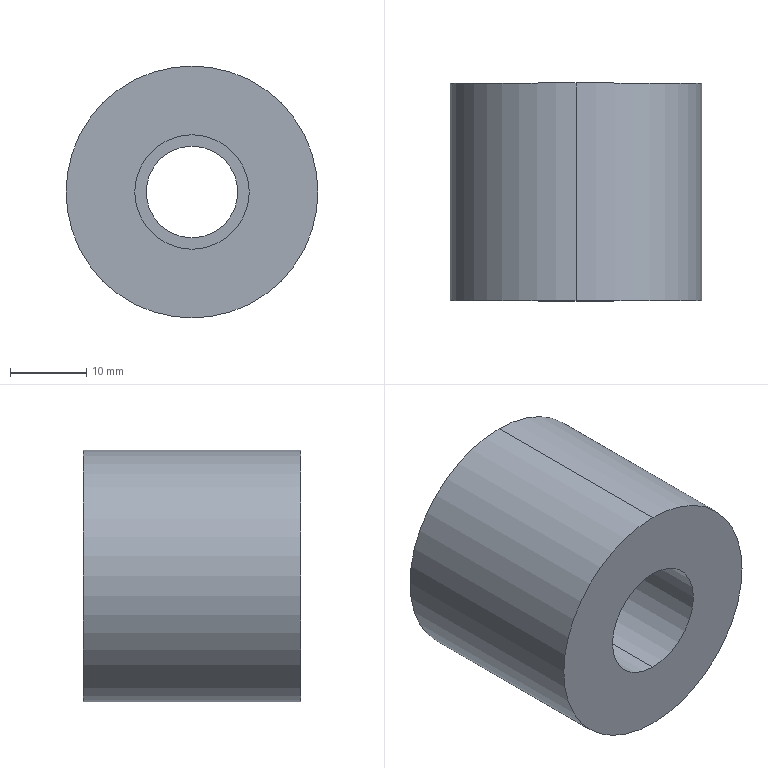Part | STEP file | PN_0065 single diaphragm coupling | 1 solid | 9 faces | box 33 x 28.5 x 33 mm | volume 20198 mm3 | cylinder 6 | plane 3 | commonest cylinder face diameters 12 x2 15 x2 33 x2
STEP:
#1=CARTESIAN_POINT('',(0.,0.,0.));
#2=DIRECTION('',(0.,0.,1.));
#3=DIRECTION('',(1.,0.,0.));
#4=AXIS2_PLACEMENT_3D('',#1,#2,#3);
#5=CARTESIAN_POINT('',(0.,15.,-7.5));
#6=VERTEX_POINT('',#5);
#7=CARTESIAN_POINT('',(0.,0.,-7.5));
#8=VERTEX_POINT('',#7);
#9=CARTESIAN_POINT('',(0.,15.,-7.5));
#10=DIRECTION('',(0.,-1.,0.));
#11=VECTOR('',#10,1.);
#12=LINE('',#9,#11);
#13=CARTESIAN_POINT('',(0.,15.,0.));
#14=DIRECTION('',(0.,-1.,0.));
#15=DIRECTION('',(0.,0.,-1.));
#16=AXIS2_PLACEMENT_3D('',#13,#14,#15);
#17=CYLINDRICAL_SURFACE('',#16,7.5);
#18=CARTESIAN_POINT('',(6.283,0.));
#19=DIRECTION('',(0.,1.));
#20=VECTOR('',#19,1.);
#21=LINE('',#18,#20);
#22=(GEOMETRIC_REPRESENTATION_CONTEXT(2)PARAMETRIC_REPRESENTATION_CONTEXT()REPRESENTATION_CONTEXT('',''));
#23=DEFINITIONAL_REPRESENTATION('',(#21),#22);
#24=PCURVE('',#17,#23);
#25=CARTESIAN_POINT('',(0.,15.,0.));
#26=DIRECTION('',(0.,-1.,0.));
#27=DIRECTION('',(0.,0.,-1.));
#28=AXIS2_PLACEMENT_3D('',#25,#26,#27);
#29=CYLINDRICAL_SURFACE('',#28,7.5);
#30=CARTESIAN_POINT('',(0.,0.));
#31=DIRECTION('',(0.,1.));
#32=VECTOR('',#31,1.);
#33=LINE('',#30,#32);
#34=(GEOMETRIC_REPRESENTATION_CONTEXT(2)PARAMETRIC_REPRESENTATION_CONTEXT()REPRESENTATION_CONTEXT('',''));
#35=DEFINITIONAL_REPRESENTATION('',(#33),#34);
#36=PCURVE('',#29,#35);
#37=SURFACE_CURVE('',#12,(#24,#36),.PCURVE_S1.);
#38=EDGE_CURVE('',#6,#8,#37,.T.);
#39=ORIENTED_EDGE('',*,*,#38,.T.);
#40=CARTESIAN_POINT('',(0.,0.,7.5));
#41=VERTEX_POINT('',#40);
#42=CARTESIAN_POINT('',(0.,0.,0.));
#43=DIRECTION('',(0.,-1.,0.));
#44=DIRECTION('',(0.,0.,-1.));
#45=AXIS2_PLACEMENT_3D('',#42,#43,#44);
#46=CIRCLE('',#45,7.5);
#47=CARTESIAN_POINT('',(0.,15.));
#48=DIRECTION('',(1.,0.));
#49=VECTOR('',#48,1.);
#50=LINE('',#47,#49);
#51=(GEOMETRIC_REPRESENTATION_CONTEXT(2)PARAMETRIC_REPRESENTATION_CONTEXT()REPRESENTATION_CONTEXT('',''));
#52=DEFINITIONAL_REPRESENTATION('',(#50),#51);
#53=PCURVE('',#17,#52);
#54=CARTESIAN_POINT('',(0.,0.,0.));
#55=DIRECTION('',(0.,1.,0.));
#56=DIRECTION('',(0.,0.,1.));
#57=AXIS2_PLACEMENT_3D('',#54,#55,#56);
#58=PLANE('',#57);
#59=CARTESIAN_POINT('',(-7.5,0.));
#60=CARTESIAN_POINT('',(-7.5,12.99));
#61=CARTESIAN_POINT('',(3.75,6.495));
#62=CARTESIAN_POINT('',(15.,0.));
#63=CARTESIAN_POINT('',(3.75,-6.495));
#64=CARTESIAN_POINT('',(-7.5,-12.99));
#65=CARTESIAN_POINT('',(-7.5,0.));
#66=(BOUNDED_CURVE()B_SPLINE_CURVE(2,(#59,#60,#61,#62,#63,#64,#65),.UNSPECIFIED.,.T.,.F.)B_SPLINE_CURVE_WITH_KNOTS((1,2,2,2,2,1),(-2.094,0.,2.094,4.189,6.283,8.378),.UNSPECIFIED.)CURVE()GEOMETRIC_REPRESENTATION_ITEM()RATIONAL_B_SPLINE_CURVE((1.,0.5,1.,0.5,1.,0.5,1.))REPRESENTATION_ITEM(''));
#67=(GEOMETRIC_REPRESENTATION_CONTEXT(2)PARAMETRIC_REPRESENTATION_CONTEXT()REPRESENTATION_CONTEXT('',''));
#68=DEFINITIONAL_REPRESENTATION('',(#66),#67);
#69=PCURVE('',#58,#68);
#70=SURFACE_CURVE('',#46,(#53,#69),.PCURVE_S1.);
#71=EDGE_CURVE('',#41,#8,#70,.T.);
#72=ORIENTED_EDGE('',*,*,#71,.F.);
#73=CARTESIAN_POINT('',(0.,15.,7.5));
#74=VERTEX_POINT('',#73);
#75=CARTESIAN_POINT('',(0.,15.,7.5));
#76=DIRECTION('',(0.,-1.,0.));
#77=VECTOR('',#76,1.);
#78=LINE('',#75,#77);
#79=CARTESIAN_POINT('',(3.142,0.));
#80=DIRECTION('',(0.,1.));
#81=VECTOR('',#80,1.);
#82=LINE('',#79,#81);
#83=(GEOMETRIC_REPRESENTATION_CONTEXT(2)PARAMETRIC_REPRESENTATION_CONTEXT()REPRESENTATION_CONTEXT('',''));
#84=DEFINITIONAL_REPRESENTATION('',(#82),#83);
#85=PCURVE('',#17,#84);
#86=CARTESIAN_POINT('',(3.142,0.));
#87=DIRECTION('',(0.,1.));
#88=VECTOR('',#87,1.);
#89=LINE('',#86,#88);
#90=(GEOMETRIC_REPRESENTATION_CONTEXT(2)PARAMETRIC_REPRESENTATION_CONTEXT()REPRESENTATION_CONTEXT('',''));
#91=DEFINITIONAL_REPRESENTATION('',(#89),#90);
#92=PCURVE('',#29,#91);
#93=SURFACE_CURVE('',#78,(#85,#92),.PCURVE_S1.);
#94=EDGE_CURVE('',#74,#41,#93,.T.);
#95=ORIENTED_EDGE('',*,*,#94,.F.);
#96=CARTESIAN_POINT('',(0.,15.,0.));
#97=DIRECTION('',(0.,-1.,0.));
#98=DIRECTION('',(0.,0.,-1.));
#99=AXIS2_PLACEMENT_3D('',#96,#97,#98);
#100=CIRCLE('',#99,7.5);
#101=CARTESIAN_POINT('',(0.,0.));
#102=DIRECTION('',(1.,0.));
#103=VECTOR('',#102,1.);
#104=LINE('',#101,#103);
#105=(GEOMETRIC_REPRESENTATION_CONTEXT(2)PARAMETRIC_REPRESENTATION_CONTEXT()REPRESENTATION_CONTEXT('',''));
#106=DEFINITIONAL_REPRESENTATION('',(#104),#105);
#107=PCURVE('',#17,#106);
#108=CARTESIAN_POINT('',(0.,15.,0.));
#109=DIRECTION('',(0.,-1.,0.));
#110=DIRECTION('',(0.,0.,-1.));
#111=AXIS2_PLACEMENT_3D('',#108,#109,#110);
#112=PLANE('',#111);
#113=CARTESIAN_POINT('',(0.,0.));
#114=DIRECTION('',(1.,0.));
#115=AXIS2_PLACEMENT_2D('',#113,#114);
#116=CIRCLE('',#115,7.5);
#117=(GEOMETRIC_REPRESENTATION_CONTEXT(2)PARAMETRIC_REPRESENTATION_CONTEXT()REPRESENTATION_CONTEXT('',''));
#118=DEFINITIONAL_REPRESENTATION('',(#116),#117);
#119=PCURVE('',#112,#118);
#120=SURFACE_CURVE('',#100,(#107,#119),.PCURVE_S1.);
#121=EDGE_CURVE('',#74,#6,#120,.T.);
#122=ORIENTED_EDGE('',*,*,#121,.T.);
#123=EDGE_LOOP('',(#39,#72,#95,#122));
#124=FACE_BOUND('',#123,.F.);
#125=ADVANCED_FACE('',(#124),#17,.F.);
#126=CARTESIAN_POINT('',(0.,28.5,16.5));
#127=VERTEX_POINT('',#126);
#128=CARTESIAN_POINT('',(0.,28.5,-16.5));
#129=VERTEX_POINT('',#128);
#130=CARTESIAN_POINT('',(0.,28.5,0.));
#131=DIRECTION('',(0.,1.,0.));
#132=DIRECTION('',(0.,0.,1.));
#133=AXIS2_PLACEMENT_3D('',#130,#131,#132);
#134=CIRCLE('',#133,16.5);
#135=CARTESIAN_POINT('',(0.,28.5,0.));
#136=DIRECTION('',(0.,-1.,0.));
#137=DIRECTION('',(0.,0.,-1.));
#138=AXIS2_PLACEMENT_3D('',#135,#136,#137);
#139=CYLINDRICAL_SURFACE('',#138,16.5);
#140=CARTESIAN_POINT('',(3.142,0.));
#141=DIRECTION('',(-1.,0.));
#142=VECTOR('',#141,1.);
#143=LINE('',#140,#142);
#144=(GEOMETRIC_REPRESENTATION_CONTEXT(2)PARAMETRIC_REPRESENTATION_CONTEXT()REPRESENTATION_CONTEXT('',''));
#145=DEFINITIONAL_REPRESENTATION('',(#143),#144);
#146=PCURVE('',#139,#145);
#147=CARTESIAN_POINT('',(0.,28.5,0.));
#148=DIRECTION('',(0.,1.,0.));
#149=DIRECTION('',(0.,0.,1.));
#150=AXIS2_PLACEMENT_3D('',#147,#148,#149);
#151=PLANE('',#150);
#152=CARTESIAN_POINT('',(0.,0.));
#153=DIRECTION('',(1.,0.));
#154=AXIS2_PLACEMENT_2D('',#152,#153);
#155=CIRCLE('',#154,16.5);
#156=(GEOMETRIC_REPRESENTATION_CONTEXT(2)PARAMETRIC_REPRESENTATION_CONTEXT()REPRESENTATION_CONTEXT('',''));
#157=DEFINITIONAL_REPRESENTATION('',(#155),#156);
#158=PCURVE('',#151,#157);
#159=SURFACE_CURVE('',#134,(#146,#158),.PCURVE_S1.);
#160=EDGE_CURVE('',#127,#129,#159,.T.);
#161=ORIENTED_EDGE('',*,*,#160,.F.);
#162=CARTESIAN_POINT('',(0.,0.,16.5));
#163=VERTEX_POINT('',#162);
#164=CARTESIAN_POINT('',(0.,28.5,16.5));
#165=DIRECTION('',(0.,-1.,0.));
#166=VECTOR('',#165,1.);
#167=LINE('',#164,#166);
#168=CARTESIAN_POINT('',(3.142,0.));
#169=DIRECTION('',(0.,1.));
#170=VECTOR('',#169,1.);
#171=LINE('',#168,#170);
#172=(GEOMETRIC_REPRESENTATION_CONTEXT(2)PARAMETRIC_REPRESENTATION_CONTEXT()REPRESENTATION_CONTEXT('',''));
#173=DEFINITIONAL_REPRESENTATION('',(#171),#172);
#174=PCURVE('',#139,#173);
#175=CARTESIAN_POINT('',(0.,28.5,0.));
#176=DIRECTION('',(0.,-1.,0.));
#177=DIRECTION('',(0.,0.,-1.));
#178=AXIS2_PLACEMENT_3D('',#175,#176,#177);
#179=CYLINDRICAL_SURFACE('',#178,16.5);
#180=CARTESIAN_POINT('',(3.142,0.));
#181=DIRECTION('',(0.,1.));
#182=VECTOR('',#181,1.);
#183=LINE('',#180,#182);
#184=(GEOMETRIC_REPRESENTATION_CONTEXT(2)PARAMETRIC_REPRESENTATION_CONTEXT()REPRESENTATION_CONTEXT('',''));
#185=DEFINITIONAL_REPRESENTATION('',(#183),#184);
#186=PCURVE('',#179,#185);
#187=SURFACE_CURVE('',#167,(#174,#186),.PCURVE_S1.);
#188=EDGE_CURVE('',#127,#163,#187,.T.);
#189=ORIENTED_EDGE('',*,*,#188,.T.);
#190=CARTESIAN_POINT('',(0.,0.,-16.5));
#191=VERTEX_POINT('',#190);
#192=CARTESIAN_POINT('',(0.,0.,0.));
#193=DIRECTION('',(0.,1.,0.));
#194=DIRECTION('',(0.,0.,1.));
#195=AXIS2_PLACEMENT_3D('',#192,#193,#194);
#196=CIRCLE('',#195,16.5);
#197=CARTESIAN_POINT('',(3.142,28.5));
#198=DIRECTION('',(-1.,0.));
#199=VECTOR('',#198,1.);
#200=LINE('',#197,#199);
#201=(GEOMETRIC_REPRESENTATION_CONTEXT(2)PARAMETRIC_REPRESENTATION_CONTEXT()REPRESENTATION_CONTEXT('',''));
#202=DEFINITIONAL_REPRESENTATION('',(#200),#201);
#203=PCURVE('',#139,#202);
#204=CARTESIAN_POINT('',(0.,0.));
#205=DIRECTION('',(1.,0.));
#206=AXIS2_PLACEMENT_2D('',#204,#205);
#207=CIRCLE('',#206,16.5);
#208=(GEOMETRIC_REPRESENTATION_CONTEXT(2)PARAMETRIC_REPRESENTATION_CONTEXT()REPRESENTATION_CONTEXT('',''));
#209=DEFINITIONAL_REPRESENTATION('',(#207),#208);
#210=PCURVE('',#58,#209);
#211=SURFACE_CURVE('',#196,(#203,#210),.PCURVE_S1.);
#212=EDGE_CURVE('',#163,#191,#211,.T.);
#213=ORIENTED_EDGE('',*,*,#212,.T.);
#214=CARTESIAN_POINT('',(0.,28.5,-16.5));
#215=DIRECTION('',(0.,-1.,0.));
#216=VECTOR('',#215,1.);
#217=LINE('',#214,#216);
#218=CARTESIAN_POINT('',(0.,0.));
#219=DIRECTION('',(0.,1.));
#220=VECTOR('',#219,1.);
#221=LINE('',#218,#220);
#222=(GEOMETRIC_REPRESENTATION_CONTEXT(2)PARAMETRIC_REPRESENTATION_CONTEXT()REPRESENTATION_CONTEXT('',''));
#223=DEFINITIONAL_REPRESENTATION('',(#221),#222);
#224=PCURVE('',#139,#223);
#225=CARTESIAN_POINT('',(6.283,0.));
#226=DIRECTION('',(0.,1.));
#227=VECTOR('',#226,1.);
#228=LINE('',#225,#227);
#229=(GEOMETRIC_REPRESENTATION_CONTEXT(2)PARAMETRIC_REPRESENTATION_CONTEXT()REPRESENTATION_CONTEXT('',''));
#230=DEFINITIONAL_REPRESENTATION('',(#228),#229);
#231=PCURVE('',#179,#230);
#232=SURFACE_CURVE('',#217,(#224,#231),.PCURVE_S1.);
#233=EDGE_CURVE('',#129,#191,#232,.T.);
#234=ORIENTED_EDGE('',*,*,#233,.F.);
#235=EDGE_LOOP('',(#161,#189,#213,#234));
#236=FACE_BOUND('',#235,.T.);
#237=ADVANCED_FACE('',(#236),#139,.T.);
#238=CARTESIAN_POINT('',(0.,15.,6.));
#239=VERTEX_POINT('',#238);
#240=CARTESIAN_POINT('',(0.,28.5,6.));
#241=VERTEX_POINT('',#240);
#242=CARTESIAN_POINT('',(0.,0.,6.));
#243=DIRECTION('',(0.,1.,0.));
#244=VECTOR('',#243,1.);
#245=LINE('',#242,#244);
#246=CARTESIAN_POINT('',(0.,0.,0.));
#247=DIRECTION('',(0.,1.,0.));
#248=DIRECTION('',(0.,0.,1.));
#249=AXIS2_PLACEMENT_3D('',#246,#247,#248);
#250=CYLINDRICAL_SURFACE('',#249,6.);
#251=CARTESIAN_POINT('',(6.283,0.));
#252=DIRECTION('',(0.,1.));
#253=VECTOR('',#252,1.);
#254=LINE('',#251,#253);
#255=(GEOMETRIC_REPRESENTATION_CONTEXT(2)PARAMETRIC_REPRESENTATION_CONTEXT()REPRESENTATION_CONTEXT('',''));
#256=DEFINITIONAL_REPRESENTATION('',(#254),#255);
#257=PCURVE('',#250,#256);
#258=CARTESIAN_POINT('',(0.,0.,0.));
#259=DIRECTION('',(0.,1.,0.));
#260=DIRECTION('',(0.,0.,1.));
#261=AXIS2_PLACEMENT_3D('',#258,#259,#260);
#262=CYLINDRICAL_SURFACE('',#261,6.);
#263=CARTESIAN_POINT('',(0.,0.));
#264=DIRECTION('',(0.,1.));
#265=VECTOR('',#264,1.);
#266=LINE('',#263,#265);
#267=(GEOMETRIC_REPRESENTATION_CONTEXT(2)PARAMETRIC_REPRESENTATION_CONTEXT()REPRESENTATION_CONTEXT('',''));
#268=DEFINITIONAL_REPRESENTATION('',(#266),#267);
#269=PCURVE('',#262,#268);
#270=SURFACE_CURVE('',#245,(#257,#269),.PCURVE_S1.);
#271=EDGE_CURVE('',#239,#241,#270,.T.);
#272=ORIENTED_EDGE('',*,*,#271,.T.);
#273=CARTESIAN_POINT('',(0.,28.5,-6.));
#274=VERTEX_POINT('',#273);
#275=CARTESIAN_POINT('',(0.,28.5,0.));
#276=DIRECTION('',(0.,1.,0.));
#277=DIRECTION('',(0.,0.,1.));
#278=AXIS2_PLACEMENT_3D('',#275,#276,#277);
#279=CIRCLE('',#278,6.);
#280=CARTESIAN_POINT('',(0.,28.5));
#281=DIRECTION('',(1.,0.));
#282=VECTOR('',#281,1.);
#283=LINE('',#280,#282);
#284=(GEOMETRIC_REPRESENTATION_CONTEXT(2)PARAMETRIC_REPRESENTATION_CONTEXT()REPRESENTATION_CONTEXT('',''));
#285=DEFINITIONAL_REPRESENTATION('',(#283),#284);
#286=PCURVE('',#250,#285);
#287=CARTESIAN_POINT('',(0.,0.));
#288=DIRECTION('',(1.,0.));
#289=AXIS2_PLACEMENT_2D('',#287,#288);
#290=CIRCLE('',#289,6.);
#291=(GEOMETRIC_REPRESENTATION_CONTEXT(2)PARAMETRIC_REPRESENTATION_CONTEXT()REPRESENTATION_CONTEXT('',''));
#292=DEFINITIONAL_REPRESENTATION('',(#290),#291);
#293=PCURVE('',#151,#292);
#294=SURFACE_CURVE('',#279,(#286,#293),.PCURVE_S1.);
#295=EDGE_CURVE('',#274,#241,#294,.T.);
#296=ORIENTED_EDGE('',*,*,#295,.F.);
#297=CARTESIAN_POINT('',(0.,15.,-6.));
#298=VERTEX_POINT('',#297);
#299=CARTESIAN_POINT('',(0.,0.,-6.));
#300=DIRECTION('',(0.,1.,0.));
#301=VECTOR('',#300,1.);
#302=LINE('',#299,#301);
#303=CARTESIAN_POINT('',(3.142,0.));
#304=DIRECTION('',(0.,1.));
#305=VECTOR('',#304,1.);
#306=LINE('',#303,#305);
#307=(GEOMETRIC_REPRESENTATION_CONTEXT(2)PARAMETRIC_REPRESENTATION_CONTEXT()REPRESENTATION_CONTEXT('',''));
#308=DEFINITIONAL_REPRESENTATION('',(#306),#307);
#309=PCURVE('',#250,#308);
#310=CARTESIAN_POINT('',(3.142,0.));
#311=DIRECTION('',(0.,1.));
#312=VECTOR('',#311,1.);
#313=LINE('',#310,#312);
#314=(GEOMETRIC_REPRESENTATION_CONTEXT(2)PARAMETRIC_REPRESENTATION_CONTEXT()REPRESENTATION_CONTEXT('',''));
#315=DEFINITIONAL_REPRESENTATION('',(#313),#314);
#316=PCURVE('',#262,#315);
#317=SURFACE_CURVE('',#302,(#309,#316),.PCURVE_S1.);
#318=EDGE_CURVE('',#298,#274,#317,.T.);
#319=ORIENTED_EDGE('',*,*,#318,.F.);
#320=CARTESIAN_POINT('',(0.,15.,0.));
#321=DIRECTION('',(0.,1.,0.));
#322=DIRECTION('',(0.,0.,-1.));
#323=AXIS2_PLACEMENT_3D('',#320,#321,#322);
#324=CIRCLE('',#323,6.);
#325=CARTESIAN_POINT('',(3.142,15.));
#326=DIRECTION('',(1.,0.));
#327=VECTOR('',#326,1.);
#328=LINE('',#325,#327);
#329=(GEOMETRIC_REPRESENTATION_CONTEXT(2)PARAMETRIC_REPRESENTATION_CONTEXT()REPRESENTATION_CONTEXT('',''));
#330=DEFINITIONAL_REPRESENTATION('',(#328),#329);
#331=PCURVE('',#250,#330);
#332=CARTESIAN_POINT('',(6.,0.));
#333=CARTESIAN_POINT('',(6.,-10.392));
#334=CARTESIAN_POINT('',(-3.,-5.196));
#335=CARTESIAN_POINT('',(-12.,0.));
#336=CARTESIAN_POINT('',(-3.,5.196));
#337=CARTESIAN_POINT('',(6.,10.392));
#338=CARTESIAN_POINT('',(6.,0.));
#339=(BOUNDED_CURVE()B_SPLINE_CURVE(2,(#332,#333,#334,#335,#336,#337,#338),.UNSPECIFIED.,.T.,.F.)B_SPLINE_CURVE_WITH_KNOTS((1,2,2,2,2,1),(-2.094,0.,2.094,4.189,6.283,8.378),.UNSPECIFIED.)CURVE()GEOMETRIC_REPRESENTATION_ITEM()RATIONAL_B_SPLINE_CURVE((1.,0.5,1.,0.5,1.,0.5,1.))REPRESENTATION_ITEM(''));
#340=(GEOMETRIC_REPRESENTATION_CONTEXT(2)PARAMETRIC_REPRESENTATION_CONTEXT()REPRESENTATION_CONTEXT('',''));
#341=DEFINITIONAL_REPRESENTATION('',(#339),#340);
#342=PCURVE('',#112,#341);
#343=SURFACE_CURVE('',#324,(#331,#342),.PCURVE_S1.);
#344=EDGE_CURVE('',#298,#239,#343,.T.);
#345=ORIENTED_EDGE('',*,*,#344,.T.);
#346=EDGE_LOOP('',(#272,#296,#319,#345));
#347=FACE_BOUND('',#346,.F.);
#348=ADVANCED_FACE('',(#347),#250,.F.);
#349=CARTESIAN_POINT('',(0.,28.5,0.));
#350=DIRECTION('',(0.,1.,0.));
#351=DIRECTION('',(0.,0.,1.));
#352=AXIS2_PLACEMENT_3D('',#349,#350,#351);
#353=CIRCLE('',#352,6.);
#354=CARTESIAN_POINT('',(0.,28.5));
#355=DIRECTION('',(1.,0.));
#356=VECTOR('',#355,1.);
#357=LINE('',#354,#356);
#358=(GEOMETRIC_REPRESENTATION_CONTEXT(2)PARAMETRIC_REPRESENTATION_CONTEXT()REPRESENTATION_CONTEXT('',''));
#359=DEFINITIONAL_REPRESENTATION('',(#357),#358);
#360=PCURVE('',#262,#359);
#361=CARTESIAN_POINT('',(0.,0.));
#362=DIRECTION('',(1.,0.));
#363=AXIS2_PLACEMENT_2D('',#361,#362);
#364=CIRCLE('',#363,6.);
#365=(GEOMETRIC_REPRESENTATION_CONTEXT(2)PARAMETRIC_REPRESENTATION_CONTEXT()REPRESENTATION_CONTEXT('',''));
#366=DEFINITIONAL_REPRESENTATION('',(#364),#365);
#367=PCURVE('',#151,#366);
#368=SURFACE_CURVE('',#353,(#360,#367),.PCURVE_S1.);
#369=EDGE_CURVE('',#241,#274,#368,.T.);
#370=ORIENTED_EDGE('',*,*,#369,.F.);
#371=ORIENTED_EDGE('',*,*,#271,.F.);
#372=CARTESIAN_POINT('',(0.,15.,0.));
#373=DIRECTION('',(0.,1.,0.));
#374=DIRECTION('',(0.,0.,-1.));
#375=AXIS2_PLACEMENT_3D('',#372,#373,#374);
#376=CIRCLE('',#375,6.);
#377=CARTESIAN_POINT('',(-3.142,15.));
#378=DIRECTION('',(1.,0.));
#379=VECTOR('',#378,1.);
#380=LINE('',#377,#379);
#381=(GEOMETRIC_REPRESENTATION_CONTEXT(2)PARAMETRIC_REPRESENTATION_CONTEXT()REPRESENTATION_CONTEXT('',''));
#382=DEFINITIONAL_REPRESENTATION('',(#380),#381);
#383=PCURVE('',#262,#382);
#384=CARTESIAN_POINT('',(6.,0.));
#385=CARTESIAN_POINT('',(6.,-10.392));
#386=CARTESIAN_POINT('',(-3.,-5.196));
#387=CARTESIAN_POINT('',(-12.,0.));
#388=CARTESIAN_POINT('',(-3.,5.196));
#389=CARTESIAN_POINT('',(6.,10.392));
#390=CARTESIAN_POINT('',(6.,0.));
#391=(BOUNDED_CURVE()B_SPLINE_CURVE(2,(#384,#385,#386,#387,#388,#389,#390),.UNSPECIFIED.,.T.,.F.)B_SPLINE_CURVE_WITH_KNOTS((1,2,2,2,2,1),(-2.094,0.,2.094,4.189,6.283,8.378),.UNSPECIFIED.)CURVE()GEOMETRIC_REPRESENTATION_ITEM()RATIONAL_B_SPLINE_CURVE((1.,0.5,1.,0.5,1.,0.5,1.))REPRESENTATION_ITEM(''));
#392=(GEOMETRIC_REPRESENTATION_CONTEXT(2)PARAMETRIC_REPRESENTATION_CONTEXT()REPRESENTATION_CONTEXT('',''));
#393=DEFINITIONAL_REPRESENTATION('',(#391),#392);
#394=PCURVE('',#112,#393);
#395=SURFACE_CURVE('',#376,(#383,#394),.PCURVE_S1.);
#396=EDGE_CURVE('',#239,#298,#395,.T.);
#397=ORIENTED_EDGE('',*,*,#396,.T.);
#398=ORIENTED_EDGE('',*,*,#318,.T.);
#399=EDGE_LOOP('',(#370,#371,#397,#398));
#400=FACE_BOUND('',#399,.F.);
#401=ADVANCED_FACE('',(#400),#262,.F.);
#402=ORIENTED_EDGE('',*,*,#188,.F.);
#403=CARTESIAN_POINT('',(0.,28.5,0.));
#404=DIRECTION('',(0.,1.,0.));
#405=DIRECTION('',(0.,0.,1.));
#406=AXIS2_PLACEMENT_3D('',#403,#404,#405);
#407=CIRCLE('',#406,16.5);
#408=CARTESIAN_POINT('',(9.425,0.));
#409=DIRECTION('',(-1.,0.));
#410=VECTOR('',#409,1.);
#411=LINE('',#408,#410);
#412=(GEOMETRIC_REPRESENTATION_CONTEXT(2)PARAMETRIC_REPRESENTATION_CONTEXT()REPRESENTATION_CONTEXT('',''));
#413=DEFINITIONAL_REPRESENTATION('',(#411),#412);
#414=PCURVE('',#179,#413);
#415=CARTESIAN_POINT('',(0.,0.));
#416=DIRECTION('',(1.,0.));
#417=AXIS2_PLACEMENT_2D('',#415,#416);
#418=CIRCLE('',#417,16.5);
#419=(GEOMETRIC_REPRESENTATION_CONTEXT(2)PARAMETRIC_REPRESENTATION_CONTEXT()REPRESENTATION_CONTEXT('',''));
#420=DEFINITIONAL_REPRESENTATION('',(#418),#419);
#421=PCURVE('',#151,#420);
#422=SURFACE_CURVE('',#407,(#414,#421),.PCURVE_S1.);
#423=EDGE_CURVE('',#129,#127,#422,.T.);
#424=ORIENTED_EDGE('',*,*,#423,.F.);
#425=ORIENTED_EDGE('',*,*,#233,.T.);
#426=CARTESIAN_POINT('',(0.,0.,0.));
#427=DIRECTION('',(0.,1.,0.));
#428=DIRECTION('',(0.,0.,1.));
#429=AXIS2_PLACEMENT_3D('',#426,#427,#428);
#430=CIRCLE('',#429,16.5);
#431=CARTESIAN_POINT('',(9.425,28.5));
#432=DIRECTION('',(-1.,0.));
#433=VECTOR('',#432,1.);
#434=LINE('',#431,#433);
#435=(GEOMETRIC_REPRESENTATION_CONTEXT(2)PARAMETRIC_REPRESENTATION_CONTEXT()REPRESENTATION_CONTEXT('',''));
#436=DEFINITIONAL_REPRESENTATION('',(#434),#435);
#437=PCURVE('',#179,#436);
#438=CARTESIAN_POINT('',(0.,0.));
#439=DIRECTION('',(1.,0.));
#440=AXIS2_PLACEMENT_2D('',#438,#439);
#441=CIRCLE('',#440,16.5);
#442=(GEOMETRIC_REPRESENTATION_CONTEXT(2)PARAMETRIC_REPRESENTATION_CONTEXT()REPRESENTATION_CONTEXT('',''));
#443=DEFINITIONAL_REPRESENTATION('',(#441),#442);
#444=PCURVE('',#58,#443);
#445=SURFACE_CURVE('',#430,(#437,#444),.PCURVE_S1.);
#446=EDGE_CURVE('',#191,#163,#445,.T.);
#447=ORIENTED_EDGE('',*,*,#446,.T.);
#448=EDGE_LOOP('',(#402,#424,#425,#447));
#449=FACE_BOUND('',#448,.T.);
#450=ADVANCED_FACE('',(#449),#179,.T.);
#451=ORIENTED_EDGE('',*,*,#369,.F.);
#452=ORIENTED_EDGE('',*,*,#295,.F.);
#453=EDGE_LOOP('',(#451,#452));
#454=FACE_BOUND('',#453,.T.);
#455=ORIENTED_EDGE('',*,*,#423,.T.);
#456=ORIENTED_EDGE('',*,*,#160,.T.);
#457=EDGE_LOOP('',(#455,#456));
#458=FACE_BOUND('',#457,.T.);
#459=ADVANCED_FACE('',(#454,#458),#151,.T.);
#460=CARTESIAN_POINT('',(0.,0.,0.));
#461=DIRECTION('',(0.,-1.,0.));
#462=DIRECTION('',(0.,0.,-1.));
#463=AXIS2_PLACEMENT_3D('',#460,#461,#462);
#464=CIRCLE('',#463,7.5);
#465=CARTESIAN_POINT('',(-7.5,0.));
#466=CARTESIAN_POINT('',(-7.5,12.99));
#467=CARTESIAN_POINT('',(3.75,6.495));
#468=CARTESIAN_POINT('',(15.,0.));
#469=CARTESIAN_POINT('',(3.75,-6.495));
#470=CARTESIAN_POINT('',(-7.5,-12.99));
#471=CARTESIAN_POINT('',(-7.5,0.));
#472=(BOUNDED_CURVE()B_SPLINE_CURVE(2,(#465,#466,#467,#468,#469,#470,#471),.UNSPECIFIED.,.T.,.F.)B_SPLINE_CURVE_WITH_KNOTS((1,2,2,2,2,1),(-2.094,0.,2.094,4.189,6.283,8.378),.UNSPECIFIED.)CURVE()GEOMETRIC_REPRESENTATION_ITEM()RATIONAL_B_SPLINE_CURVE((1.,0.5,1.,0.5,1.,0.5,1.))REPRESENTATION_ITEM(''));
#473=(GEOMETRIC_REPRESENTATION_CONTEXT(2)PARAMETRIC_REPRESENTATION_CONTEXT()REPRESENTATION_CONTEXT('',''));
#474=DEFINITIONAL_REPRESENTATION('',(#472),#473);
#475=PCURVE('',#58,#474);
#476=CARTESIAN_POINT('',(0.,15.));
#477=DIRECTION('',(1.,0.));
#478=VECTOR('',#477,1.);
#479=LINE('',#476,#478);
#480=(GEOMETRIC_REPRESENTATION_CONTEXT(2)PARAMETRIC_REPRESENTATION_CONTEXT()REPRESENTATION_CONTEXT('',''));
#481=DEFINITIONAL_REPRESENTATION('',(#479),#480);
#482=PCURVE('',#29,#481);
#483=SURFACE_CURVE('',#464,(#475,#482),.PCURVE_S1.);
#484=EDGE_CURVE('',#8,#41,#483,.T.);
#485=ORIENTED_EDGE('',*,*,#484,.F.);
#486=ORIENTED_EDGE('',*,*,#71,.F.);
#487=EDGE_LOOP('',(#485,#486));
#488=FACE_BOUND('',#487,.T.);
#489=ORIENTED_EDGE('',*,*,#446,.F.);
#490=ORIENTED_EDGE('',*,*,#212,.F.);
#491=EDGE_LOOP('',(#489,#490));
#492=FACE_BOUND('',#491,.T.);
#493=ADVANCED_FACE('',(#488,#492),#58,.F.);
#494=CARTESIAN_POINT('',(0.,15.,0.));
#495=DIRECTION('',(0.,-1.,0.));
#496=DIRECTION('',(0.,0.,-1.));
#497=AXIS2_PLACEMENT_3D('',#494,#495,#496);
#498=CIRCLE('',#497,7.5);
#499=CARTESIAN_POINT('',(0.,0.));
#500=DIRECTION('',(1.,0.));
#501=AXIS2_PLACEMENT_2D('',#499,#500);
#502=CIRCLE('',#501,7.5);
#503=(GEOMETRIC_REPRESENTATION_CONTEXT(2)PARAMETRIC_REPRESENTATION_CONTEXT()REPRESENTATION_CONTEXT('',''));
#504=DEFINITIONAL_REPRESENTATION('',(#502),#503);
#505=PCURVE('',#112,#504);
#506=CARTESIAN_POINT('',(0.,0.));
#507=DIRECTION('',(1.,0.));
#508=VECTOR('',#507,1.);
#509=LINE('',#506,#508);
#510=(GEOMETRIC_REPRESENTATION_CONTEXT(2)PARAMETRIC_REPRESENTATION_CONTEXT()REPRESENTATION_CONTEXT('',''));
#511=DEFINITIONAL_REPRESENTATION('',(#509),#510);
#512=PCURVE('',#29,#511);
#513=SURFACE_CURVE('',#498,(#505,#512),.PCURVE_S1.);
#514=EDGE_CURVE('',#6,#74,#513,.T.);
#515=ORIENTED_EDGE('',*,*,#514,.T.);
#516=ORIENTED_EDGE('',*,*,#121,.T.);
#517=EDGE_LOOP('',(#515,#516));
#518=FACE_BOUND('',#517,.T.);
#519=ORIENTED_EDGE('',*,*,#396,.T.);
#520=ORIENTED_EDGE('',*,*,#344,.T.);
#521=EDGE_LOOP('',(#519,#520));
#522=FACE_BOUND('',#521,.T.);
#523=ADVANCED_FACE('',(#518,#522),#112,.T.);
#524=ORIENTED_EDGE('',*,*,#484,.F.);
#525=ORIENTED_EDGE('',*,*,#38,.F.);
#526=ORIENTED_EDGE('',*,*,#514,.T.);
#527=ORIENTED_EDGE('',*,*,#94,.T.);
#528=EDGE_LOOP('',(#524,#525,#526,#527));
#529=FACE_BOUND('',#528,.F.);
#530=ADVANCED_FACE('',(#529),#29,.F.);
#531=CLOSED_SHELL('',(#125,#237,#348,#401,#450,#459,#493,#523,#530));
#532=MANIFOLD_SOLID_BREP('',#531);
#533=(LENGTH_UNIT()NAMED_UNIT(*)SI_UNIT(.MILLI.,.METRE.));
#534=UNCERTAINTY_MEASURE_WITH_UNIT(LENGTH_MEASURE(0.0000001),#533,'','');
#535=(NAMED_UNIT(*)PLANE_ANGLE_UNIT()SI_UNIT($,.RADIAN.));
#536=(NAMED_UNIT(*)SI_UNIT($,.STERADIAN.)SOLID_ANGLE_UNIT());
#537=(GEOMETRIC_REPRESENTATION_CONTEXT(3)GLOBAL_UNCERTAINTY_ASSIGNED_CONTEXT((#534))GLOBAL_UNIT_ASSIGNED_CONTEXT((#533,#535,#536))REPRESENTATION_CONTEXT('',''));
#538=ADVANCED_BREP_SHAPE_REPRESENTATION('',(#4,#532),#537);